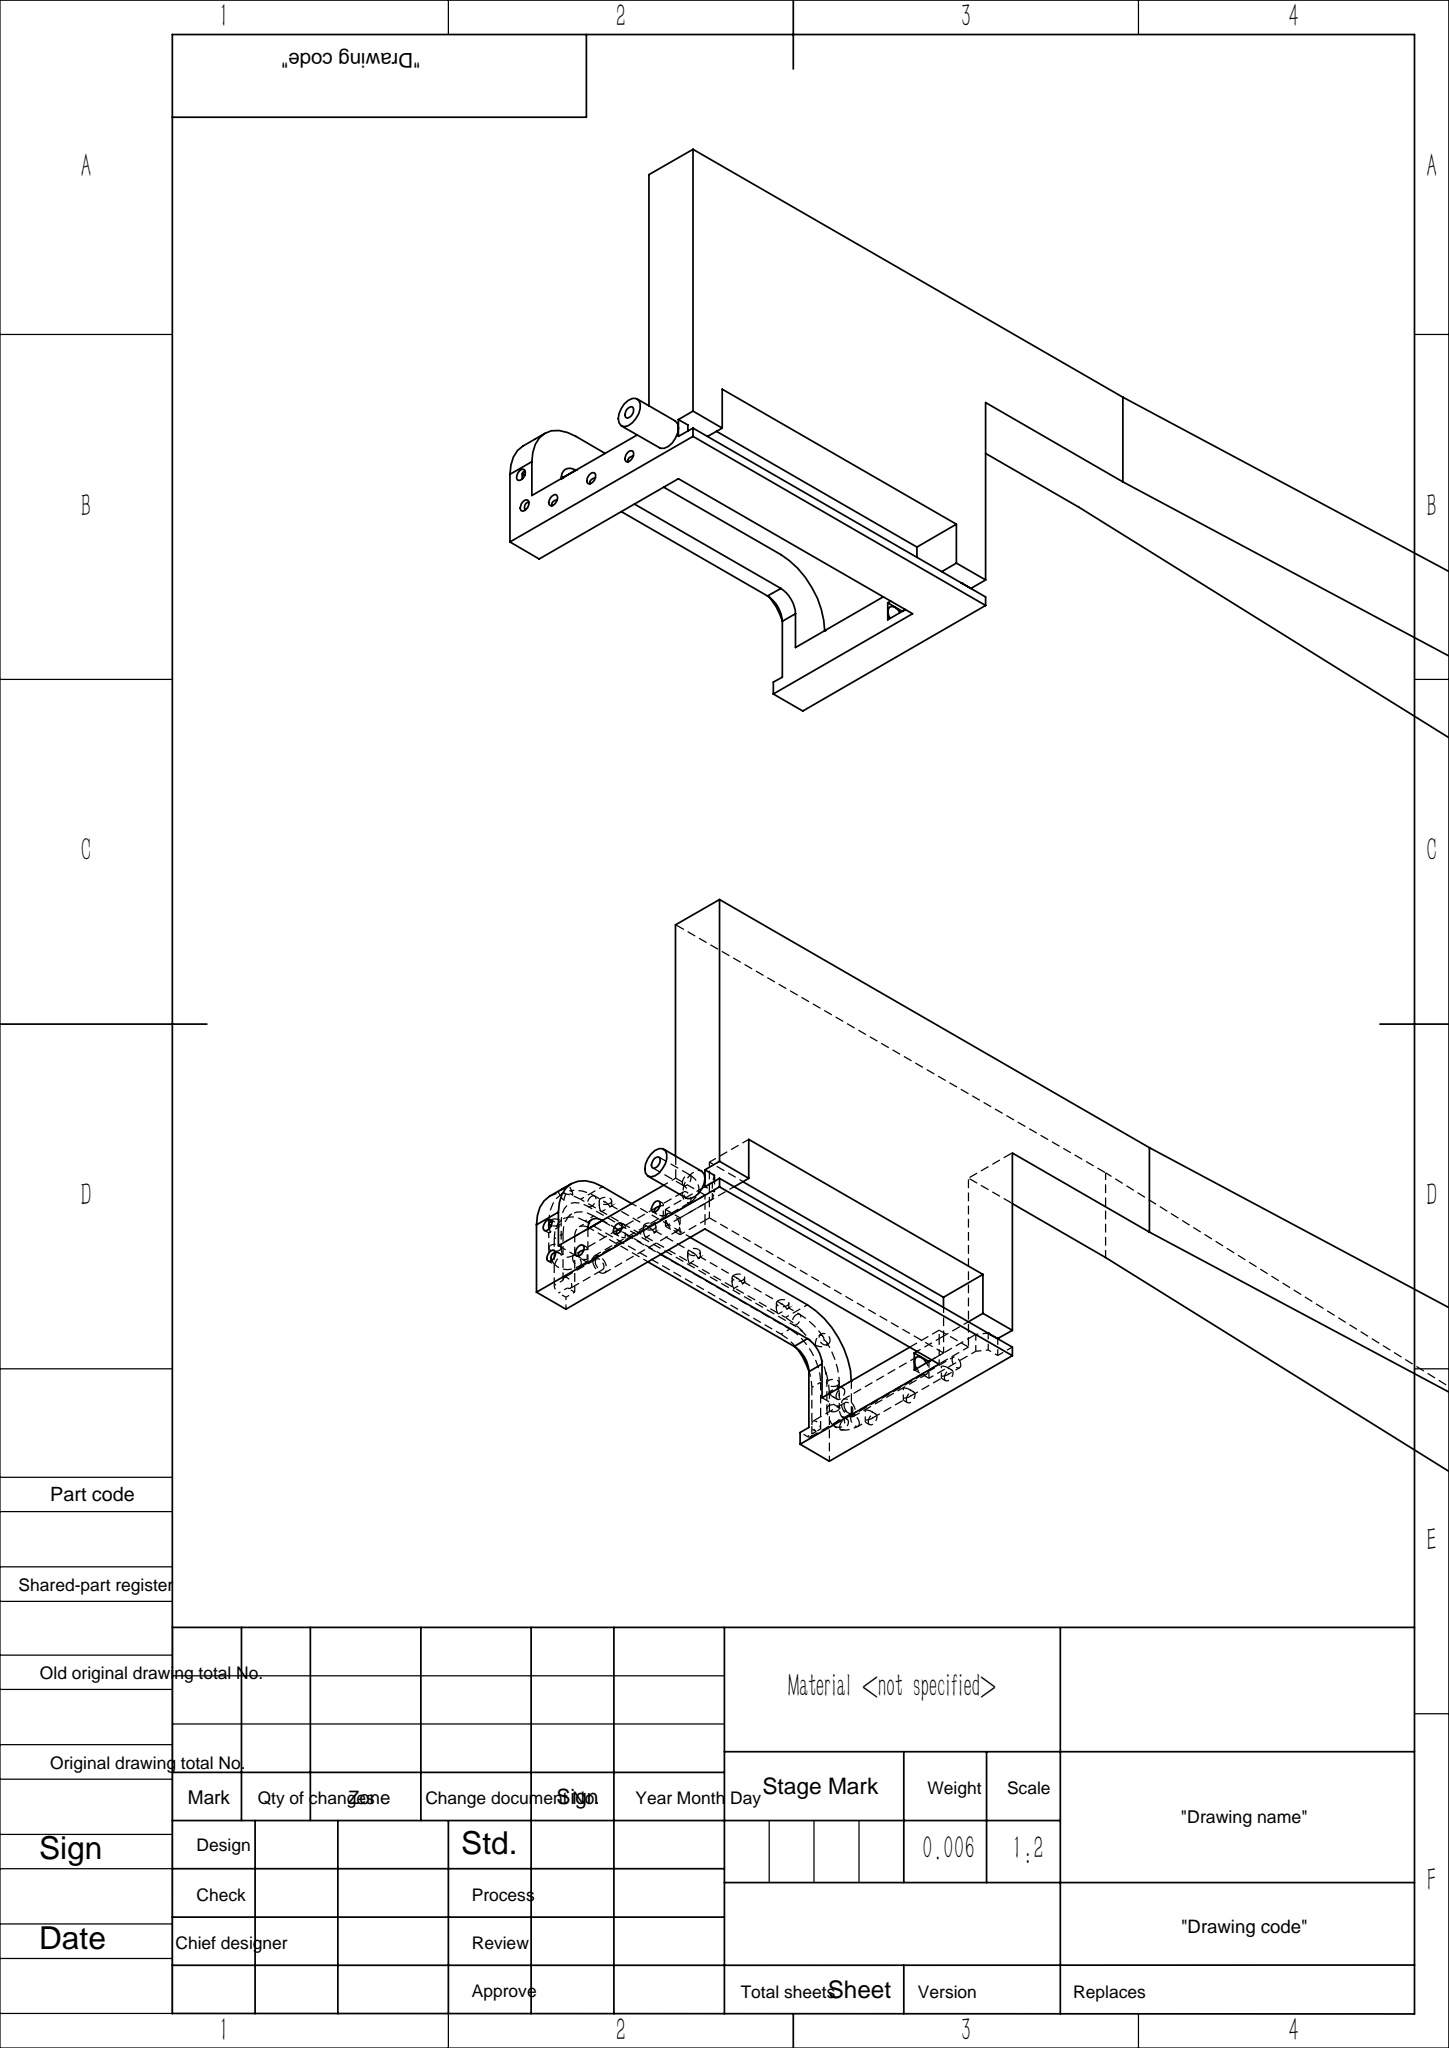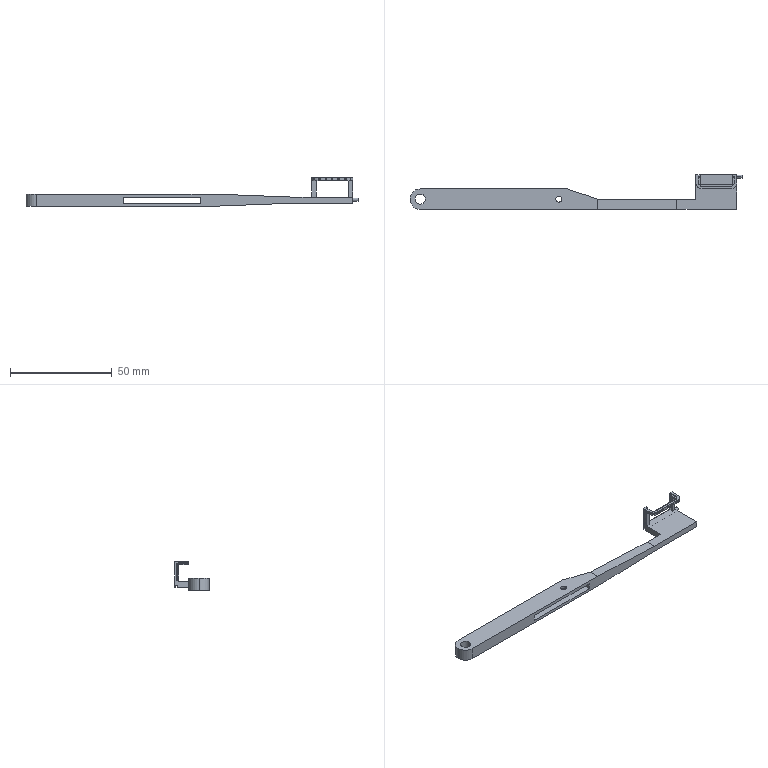Part | SolidWorks | features MirrorStock 1 | 1 solid | 142 faces | box 162.952 x 17 x 14 mm | volume 5991 mm3 | cylinder 79 | plane 53 | torus 10 | commonest cylinder face diameters 0.6 x57 0.96 x4 3 x4 0.61 x2 1.5 x2 2 x2